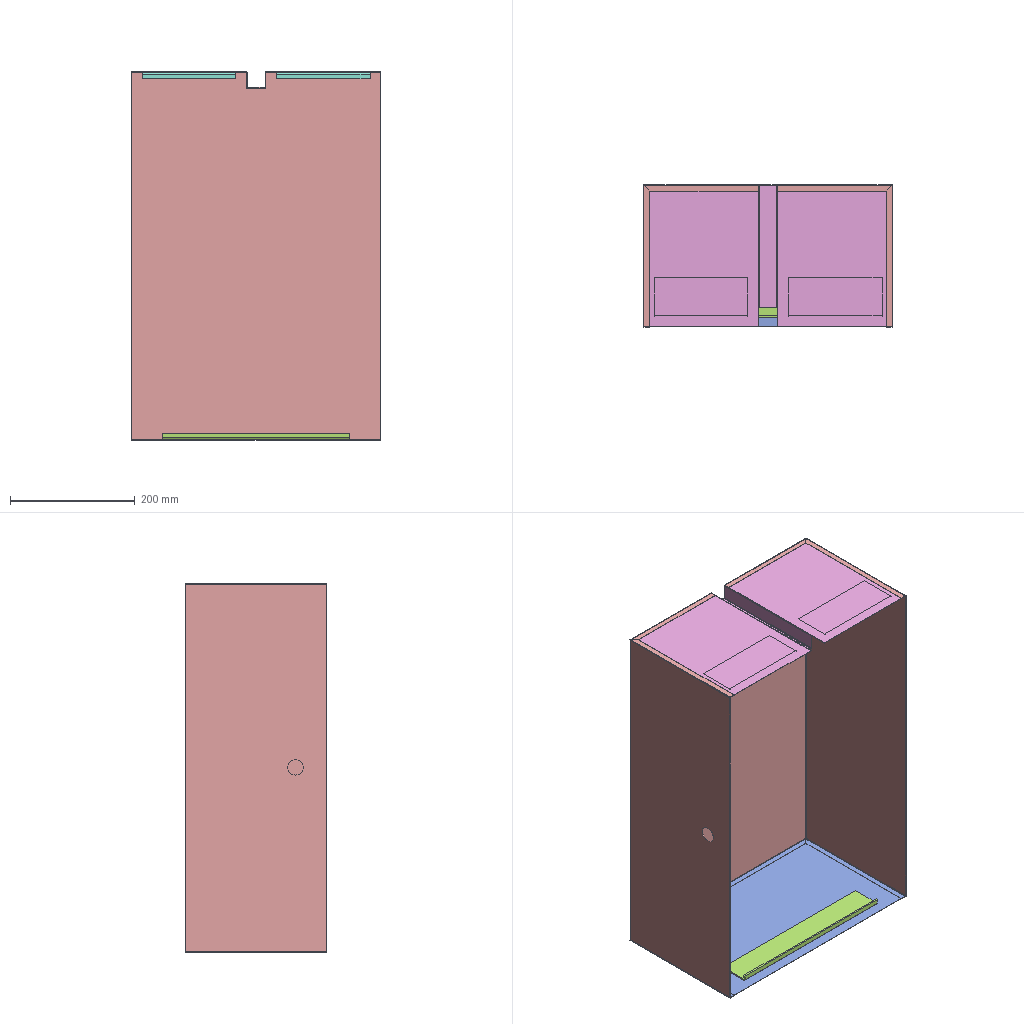Assembly | SolidWorks | 7 different items | 8 placed | box 400 x 227 x 590 mm
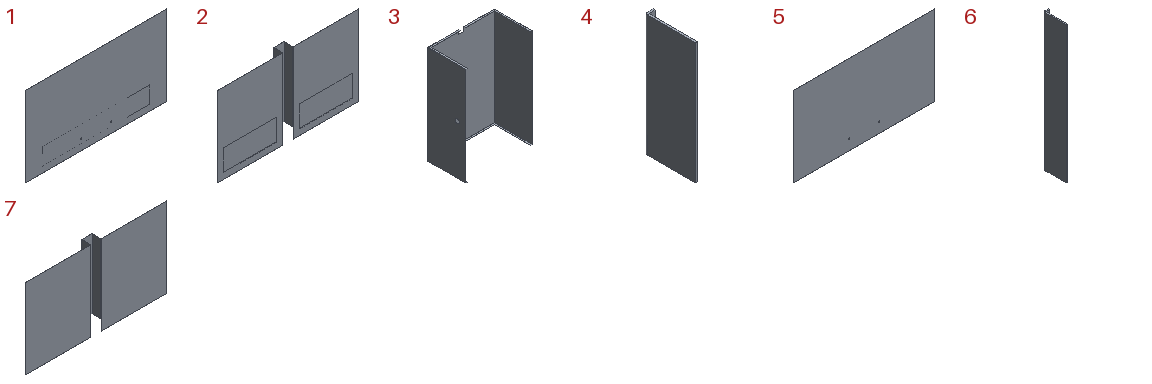Parts list (item | name | quantity | parent item | size | volume | features):
1 | (subassembly) | x1 | - | 398 x 10.5 x 226 mm | 87581 mm3 | -
2 | (subassembly) | x1 | - | 399 x 26 x 226 mm | 101592 mm3 | features LocalLPattern 1, ReferencePattern 1
3 | - | x1 | - | 399.5 x 227 x 590 mm | 258240 mm3 | features EdgeFlange 2, ICE 2, FlatPattern 1, SMBaseFlange 1, SheetMetal 1
4 | - | x2 | in 2 | 10 x 62.5 x 150 mm | 26033 mm3 | features FlatPattern 1, SMBaseFlange 1, SheetMetal 1
5 | - | x1 | in 1 | 398 x 0.5 x 226 mm | 44966 mm3 | features 3DProfileFeature 1, FlatPattern 1, HoleWzd 1, SMBaseFlange 1, SheetMetal 1
6 | - | x1 | in 1 | 10 x 49.9 x 300 mm | 42615 mm3 | features FlatPattern 1, SMBaseFlange 1, SheetMetal 1
7 | - | x1 | in 2 | 399 x 26 x 226 mm | 49527 mm3 | features FlatPattern 1, ICE 1, SMBaseFlange 1, SheetMetal 1
Mates (type | each side: item.copy, entity, surface, feature):
In the top assembly
Coincident | 3.1 face plane Edge-Flange1 | 7.1 face plane Base-Flange1
Coincident | 3.1 face plane Base-Flange1 | 7.1 face plane Base-Flange1 | 2 times
Coincident | 3.1 face plane Edge-Flange2 | 5.1 face plane Base-Flange1
Coincident | 3.1 face plane Base-Flange1 | 5.1 face plane Base-Flange1 | 2 times
In subassembly 1
Coincident | 5.2 face plane Base-Flange1 | 6.1 face plane Base-Flange1
DistanceDim | 6.1 face plane Base-Flange1 | 5.2 face plane Base-Flange1
DistanceDim | 6.1 face plane Base-Flange1 | 5.2 edge
In subassembly 2
DistanceDim | 4.1 face plane Base-Flange1 | 7.2 face plane Base-Flange1 | 2 times
Coincident | 7.2 face plane Base-Flange1 | 4.1 face plane Base-Flange1